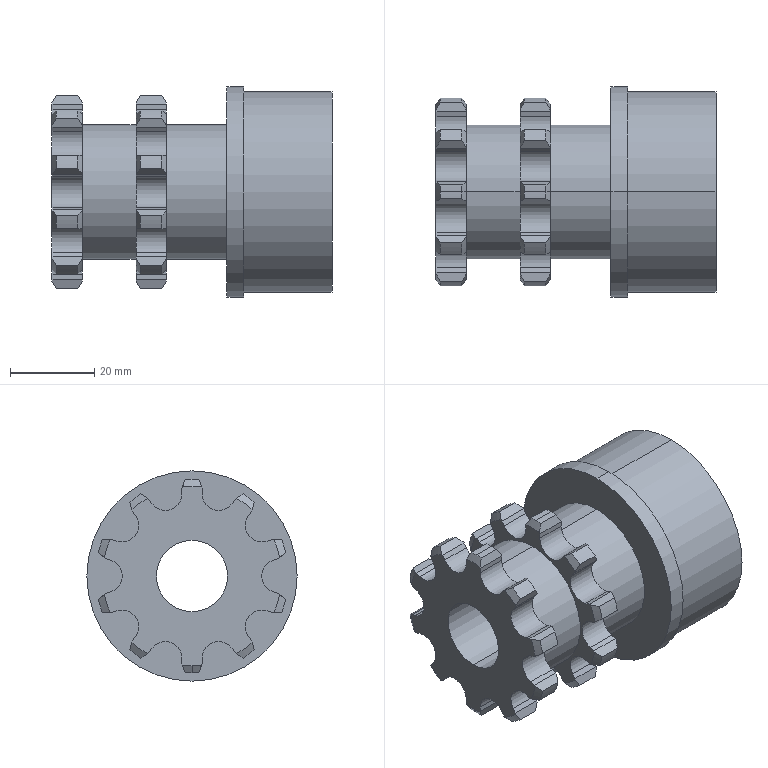Part | SolidWorks | features BaseBody 1 | 1 solid | 183 faces | box 66.6 x 50 x 50 mm | volume 69019 mm3 | plane 87 | cylinder 52 | cone 44 | commonest cylinder face diameters 46 x22 7.92 x20 32 x4 17 x2 47.6 x2 50 x2